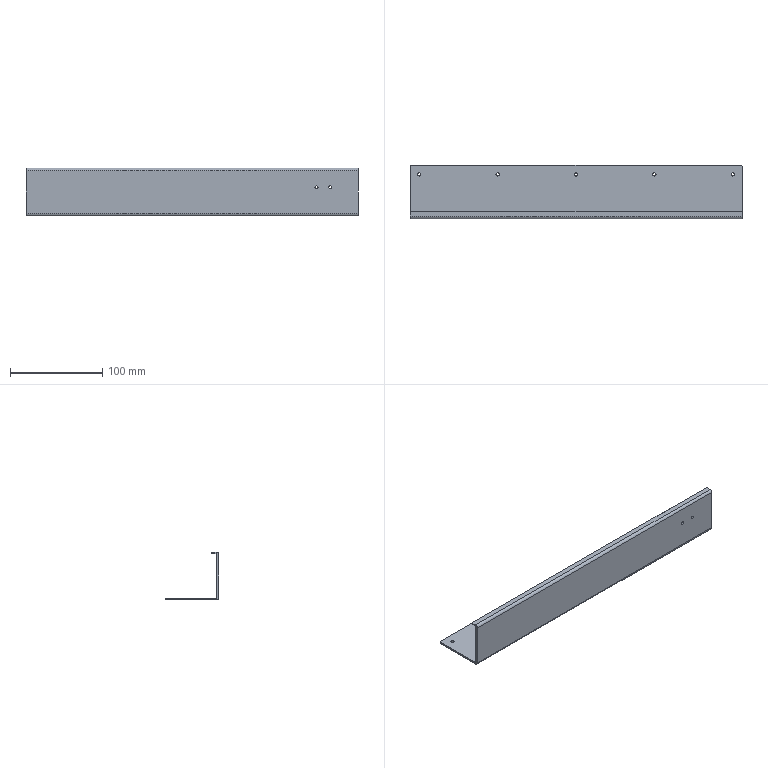Part | NX | features BREP 1 | 1 solid | 40 faces | box 360 x 58 x 52 mm | volume 80872 mm3 | plane 22 | cylinder 18 | commonest cylinder face diameters 3.5 x10 3.3 x4 1.473 x2 5.473 x2
STEP:
#1=CARTESIAN_POINT('',(135.,-2.,3.35));
#2=VERTEX_POINT('',#1);
#3=CARTESIAN_POINT('',(135.,-2.,6.65));
#4=VERTEX_POINT('',#3);
#5=CARTESIAN_POINT('',(135.,-2.,5.));
#6=DIRECTION('',(0.,1.,0.));
#7=DIRECTION('',(0.,0.,1.));
#8=AXIS2_PLACEMENT_3D('',#5,#6,#7);
#9=CIRCLE('',#8,1.65);
#10=EDGE_CURVE('',#2,#4,#9,.T.);
#11=ORIENTED_EDGE('',*,*,#10,.F.);
#12=CARTESIAN_POINT('',(135.,0.,3.35));
#13=VERTEX_POINT('',#12);
#14=CARTESIAN_POINT('',(135.,0.,3.35));
#15=DIRECTION('',(0.,1.,0.));
#16=VECTOR('',#15,1000.);
#17=LINE('',#14,#16);
#18=EDGE_CURVE('',#13,#2,#17,.F.);
#19=ORIENTED_EDGE('',*,*,#18,.F.);
#20=CARTESIAN_POINT('',(135.,0.,6.65));
#21=VERTEX_POINT('',#20);
#22=CARTESIAN_POINT('',(135.,0.,5.));
#23=DIRECTION('',(0.,1.,0.));
#24=DIRECTION('',(0.,0.,1.));
#25=AXIS2_PLACEMENT_3D('',#22,#23,#24);
#26=CIRCLE('',#25,1.65);
#27=EDGE_CURVE('',#13,#21,#26,.T.);
#28=ORIENTED_EDGE('',*,*,#27,.T.);
#29=CARTESIAN_POINT('',(135.,0.,6.65));
#30=DIRECTION('',(0.,1.,0.));
#31=VECTOR('',#30,1000.);
#32=LINE('',#29,#31);
#33=EDGE_CURVE('',#21,#4,#32,.F.);
#34=ORIENTED_EDGE('',*,*,#33,.T.);
#35=EDGE_LOOP('',(#11,#19,#28,#34));
#36=FACE_BOUND('',#35,.T.);
#37=CARTESIAN_POINT('',(135.,0.,5.));
#38=DIRECTION('',(0.,1.,0.));
#39=DIRECTION('',(0.,0.,1.));
#40=AXIS2_PLACEMENT_3D('',#37,#38,#39);
#41=CYLINDRICAL_SURFACE('',#40,1.65);
#42=ADVANCED_FACE('',(#36),#41,.F.);
#43=CARTESIAN_POINT('',(150.,-2.,3.35));
#44=VERTEX_POINT('',#43);
#45=CARTESIAN_POINT('',(150.,-2.,6.65));
#46=VERTEX_POINT('',#45);
#47=CARTESIAN_POINT('',(150.,-2.,5.));
#48=DIRECTION('',(0.,1.,0.));
#49=DIRECTION('',(0.,0.,1.));
#50=AXIS2_PLACEMENT_3D('',#47,#48,#49);
#51=CIRCLE('',#50,1.65);
#52=EDGE_CURVE('',#44,#46,#51,.T.);
#53=ORIENTED_EDGE('',*,*,#52,.F.);
#54=CARTESIAN_POINT('',(150.,0.,3.35));
#55=VERTEX_POINT('',#54);
#56=CARTESIAN_POINT('',(150.,0.,3.35));
#57=DIRECTION('',(0.,1.,0.));
#58=VECTOR('',#57,1000.);
#59=LINE('',#56,#58);
#60=EDGE_CURVE('',#55,#44,#59,.F.);
#61=ORIENTED_EDGE('',*,*,#60,.F.);
#62=CARTESIAN_POINT('',(150.,0.,6.65));
#63=VERTEX_POINT('',#62);
#64=CARTESIAN_POINT('',(150.,0.,5.));
#65=DIRECTION('',(0.,1.,0.));
#66=DIRECTION('',(0.,0.,1.));
#67=AXIS2_PLACEMENT_3D('',#64,#65,#66);
#68=CIRCLE('',#67,1.65);
#69=EDGE_CURVE('',#55,#63,#68,.T.);
#70=ORIENTED_EDGE('',*,*,#69,.T.);
#71=CARTESIAN_POINT('',(150.,0.,6.65));
#72=DIRECTION('',(0.,1.,0.));
#73=VECTOR('',#72,1000.);
#74=LINE('',#71,#73);
#75=EDGE_CURVE('',#63,#46,#74,.F.);
#76=ORIENTED_EDGE('',*,*,#75,.T.);
#77=EDGE_LOOP('',(#53,#61,#70,#76));
#78=FACE_BOUND('',#77,.T.);
#79=CARTESIAN_POINT('',(150.,0.,5.));
#80=DIRECTION('',(0.,1.,0.));
#81=DIRECTION('',(0.,0.,1.));
#82=AXIS2_PLACEMENT_3D('',#79,#80,#81);
#83=CYLINDRICAL_SURFACE('',#82,1.65);
#84=ADVANCED_FACE('',(#78),#83,.F.);
#85=CARTESIAN_POINT('',(-86.75,46.,-26.));
#86=VERTEX_POINT('',#85);
#87=CARTESIAN_POINT('',(-83.25,46.,-26.));
#88=VERTEX_POINT('',#87);
#89=CARTESIAN_POINT('',(-85.,46.,-26.));
#90=DIRECTION('',(0.,0.,1.));
#91=DIRECTION('',(0.,-1.,0.));
#92=AXIS2_PLACEMENT_3D('',#89,#90,#91);
#93=CIRCLE('',#92,1.75);
#94=EDGE_CURVE('',#86,#88,#93,.T.);
#95=ORIENTED_EDGE('',*,*,#94,.F.);
#96=CARTESIAN_POINT('',(-86.75,46.,-24.));
#97=VERTEX_POINT('',#96);
#98=CARTESIAN_POINT('',(-86.75,46.,-24.));
#99=DIRECTION('',(0.,0.,1.));
#100=VECTOR('',#99,1000.);
#101=LINE('',#98,#100);
#102=EDGE_CURVE('',#97,#86,#101,.F.);
#103=ORIENTED_EDGE('',*,*,#102,.F.);
#104=CARTESIAN_POINT('',(-83.25,46.,-24.));
#105=VERTEX_POINT('',#104);
#106=CARTESIAN_POINT('',(-85.,46.,-24.));
#107=DIRECTION('',(0.,0.,1.));
#108=DIRECTION('',(1.,0.,0.));
#109=AXIS2_PLACEMENT_3D('',#106,#107,#108);
#110=CIRCLE('',#109,1.75);
#111=EDGE_CURVE('',#97,#105,#110,.T.);
#112=ORIENTED_EDGE('',*,*,#111,.T.);
#113=CARTESIAN_POINT('',(-83.25,46.,-24.));
#114=DIRECTION('',(0.,0.,1.));
#115=VECTOR('',#114,1000.);
#116=LINE('',#113,#115);
#117=EDGE_CURVE('',#105,#88,#116,.F.);
#118=ORIENTED_EDGE('',*,*,#117,.T.);
#119=EDGE_LOOP('',(#95,#103,#112,#118));
#120=FACE_BOUND('',#119,.T.);
#121=CARTESIAN_POINT('',(-85.,46.,-24.));
#122=DIRECTION('',(0.,0.,1.));
#123=DIRECTION('',(1.,0.,0.));
#124=AXIS2_PLACEMENT_3D('',#121,#122,#123);
#125=CYLINDRICAL_SURFACE('',#124,1.75);
#126=ADVANCED_FACE('',(#120),#125,.F.);
#127=CARTESIAN_POINT('',(-1.75,46.,-26.));
#128=VERTEX_POINT('',#127);
#129=CARTESIAN_POINT('',(1.75,46.,-26.));
#130=VERTEX_POINT('',#129);
#131=CARTESIAN_POINT('',(0.,46.,-26.));
#132=DIRECTION('',(0.,0.,1.));
#133=DIRECTION('',(0.,-1.,0.));
#134=AXIS2_PLACEMENT_3D('',#131,#132,#133);
#135=CIRCLE('',#134,1.75);
#136=EDGE_CURVE('',#128,#130,#135,.T.);
#137=ORIENTED_EDGE('',*,*,#136,.F.);
#138=CARTESIAN_POINT('',(-1.75,46.,-24.));
#139=VERTEX_POINT('',#138);
#140=CARTESIAN_POINT('',(-1.75,46.,-24.));
#141=DIRECTION('',(0.,0.,1.));
#142=VECTOR('',#141,1000.);
#143=LINE('',#140,#142);
#144=EDGE_CURVE('',#139,#128,#143,.F.);
#145=ORIENTED_EDGE('',*,*,#144,.F.);
#146=CARTESIAN_POINT('',(1.75,46.,-24.));
#147=VERTEX_POINT('',#146);
#148=CARTESIAN_POINT('',(0.,46.,-24.));
#149=DIRECTION('',(0.,0.,1.));
#150=DIRECTION('',(1.,0.,0.));
#151=AXIS2_PLACEMENT_3D('',#148,#149,#150);
#152=CIRCLE('',#151,1.75);
#153=EDGE_CURVE('',#139,#147,#152,.T.);
#154=ORIENTED_EDGE('',*,*,#153,.T.);
#155=CARTESIAN_POINT('',(1.75,46.,-24.));
#156=DIRECTION('',(0.,0.,1.));
#157=VECTOR('',#156,1000.);
#158=LINE('',#155,#157);
#159=EDGE_CURVE('',#147,#130,#158,.F.);
#160=ORIENTED_EDGE('',*,*,#159,.T.);
#161=EDGE_LOOP('',(#137,#145,#154,#160));
#162=FACE_BOUND('',#161,.T.);
#163=CARTESIAN_POINT('',(0.,46.,-24.));
#164=DIRECTION('',(0.,0.,1.));
#165=DIRECTION('',(1.,0.,0.));
#166=AXIS2_PLACEMENT_3D('',#163,#164,#165);
#167=CYLINDRICAL_SURFACE('',#166,1.75);
#168=ADVANCED_FACE('',(#162),#167,.F.);
#169=CARTESIAN_POINT('',(83.25,46.,-26.));
#170=VERTEX_POINT('',#169);
#171=CARTESIAN_POINT('',(86.75,46.,-26.));
#172=VERTEX_POINT('',#171);
#173=CARTESIAN_POINT('',(85.,46.,-26.));
#174=DIRECTION('',(0.,0.,1.));
#175=DIRECTION('',(0.,-1.,0.));
#176=AXIS2_PLACEMENT_3D('',#173,#174,#175);
#177=CIRCLE('',#176,1.75);
#178=EDGE_CURVE('',#170,#172,#177,.T.);
#179=ORIENTED_EDGE('',*,*,#178,.F.);
#180=CARTESIAN_POINT('',(83.25,46.,-24.));
#181=VERTEX_POINT('',#180);
#182=CARTESIAN_POINT('',(83.25,46.,-24.));
#183=DIRECTION('',(0.,0.,1.));
#184=VECTOR('',#183,1000.);
#185=LINE('',#182,#184);
#186=EDGE_CURVE('',#181,#170,#185,.F.);
#187=ORIENTED_EDGE('',*,*,#186,.F.);
#188=CARTESIAN_POINT('',(86.75,46.,-24.));
#189=VERTEX_POINT('',#188);
#190=CARTESIAN_POINT('',(85.,46.,-24.));
#191=DIRECTION('',(0.,0.,1.));
#192=DIRECTION('',(1.,0.,0.));
#193=AXIS2_PLACEMENT_3D('',#190,#191,#192);
#194=CIRCLE('',#193,1.75);
#195=EDGE_CURVE('',#181,#189,#194,.T.);
#196=ORIENTED_EDGE('',*,*,#195,.T.);
#197=CARTESIAN_POINT('',(86.75,46.,-24.));
#198=DIRECTION('',(0.,0.,1.));
#199=VECTOR('',#198,1000.);
#200=LINE('',#197,#199);
#201=EDGE_CURVE('',#189,#172,#200,.F.);
#202=ORIENTED_EDGE('',*,*,#201,.T.);
#203=EDGE_LOOP('',(#179,#187,#196,#202));
#204=FACE_BOUND('',#203,.T.);
#205=CARTESIAN_POINT('',(85.,46.,-24.));
#206=DIRECTION('',(0.,0.,1.));
#207=DIRECTION('',(1.,0.,0.));
#208=AXIS2_PLACEMENT_3D('',#205,#206,#207);
#209=CYLINDRICAL_SURFACE('',#208,1.75);
#210=ADVANCED_FACE('',(#204),#209,.F.);
#211=CARTESIAN_POINT('',(168.25,46.,-26.));
#212=VERTEX_POINT('',#211);
#213=CARTESIAN_POINT('',(171.75,46.,-26.));
#214=VERTEX_POINT('',#213);
#215=CARTESIAN_POINT('',(170.,46.,-26.));
#216=DIRECTION('',(0.,0.,1.));
#217=DIRECTION('',(0.,-1.,0.));
#218=AXIS2_PLACEMENT_3D('',#215,#216,#217);
#219=CIRCLE('',#218,1.75);
#220=EDGE_CURVE('',#212,#214,#219,.T.);
#221=ORIENTED_EDGE('',*,*,#220,.F.);
#222=CARTESIAN_POINT('',(168.25,46.,-24.));
#223=VERTEX_POINT('',#222);
#224=CARTESIAN_POINT('',(168.25,46.,-24.));
#225=DIRECTION('',(0.,0.,1.));
#226=VECTOR('',#225,1000.);
#227=LINE('',#224,#226);
#228=EDGE_CURVE('',#223,#212,#227,.F.);
#229=ORIENTED_EDGE('',*,*,#228,.F.);
#230=CARTESIAN_POINT('',(171.75,46.,-24.));
#231=VERTEX_POINT('',#230);
#232=CARTESIAN_POINT('',(170.,46.,-24.));
#233=DIRECTION('',(0.,0.,1.));
#234=DIRECTION('',(1.,0.,0.));
#235=AXIS2_PLACEMENT_3D('',#232,#233,#234);
#236=CIRCLE('',#235,1.75);
#237=EDGE_CURVE('',#223,#231,#236,.T.);
#238=ORIENTED_EDGE('',*,*,#237,.T.);
#239=CARTESIAN_POINT('',(171.75,46.,-24.));
#240=DIRECTION('',(0.,0.,1.));
#241=VECTOR('',#240,1000.);
#242=LINE('',#239,#241);
#243=EDGE_CURVE('',#231,#214,#242,.F.);
#244=ORIENTED_EDGE('',*,*,#243,.T.);
#245=EDGE_LOOP('',(#221,#229,#238,#244));
#246=FACE_BOUND('',#245,.T.);
#247=CARTESIAN_POINT('',(170.,46.,-24.));
#248=DIRECTION('',(0.,0.,1.));
#249=DIRECTION('',(1.,0.,0.));
#250=AXIS2_PLACEMENT_3D('',#247,#248,#249);
#251=CYLINDRICAL_SURFACE('',#250,1.75);
#252=ADVANCED_FACE('',(#246),#251,.F.);
#253=CARTESIAN_POINT('',(-171.75,46.,-26.));
#254=VERTEX_POINT('',#253);
#255=CARTESIAN_POINT('',(-168.25,46.,-26.));
#256=VERTEX_POINT('',#255);
#257=CARTESIAN_POINT('',(-170.,46.,-26.));
#258=DIRECTION('',(0.,0.,1.));
#259=DIRECTION('',(0.,-1.,0.));
#260=AXIS2_PLACEMENT_3D('',#257,#258,#259);
#261=CIRCLE('',#260,1.75);
#262=EDGE_CURVE('',#254,#256,#261,.T.);
#263=ORIENTED_EDGE('',*,*,#262,.F.);
#264=CARTESIAN_POINT('',(-171.75,46.,-24.));
#265=VERTEX_POINT('',#264);
#266=CARTESIAN_POINT('',(-171.75,46.,-24.));
#267=DIRECTION('',(0.,0.,1.));
#268=VECTOR('',#267,1000.);
#269=LINE('',#266,#268);
#270=EDGE_CURVE('',#265,#254,#269,.F.);
#271=ORIENTED_EDGE('',*,*,#270,.F.);
#272=CARTESIAN_POINT('',(-168.25,46.,-24.));
#273=VERTEX_POINT('',#272);
#274=CARTESIAN_POINT('',(-170.,46.,-24.));
#275=DIRECTION('',(0.,0.,1.));
#276=DIRECTION('',(1.,0.,0.));
#277=AXIS2_PLACEMENT_3D('',#274,#275,#276);
#278=CIRCLE('',#277,1.75);
#279=EDGE_CURVE('',#265,#273,#278,.T.);
#280=ORIENTED_EDGE('',*,*,#279,.T.);
#281=CARTESIAN_POINT('',(-168.25,46.,-24.));
#282=DIRECTION('',(0.,0.,1.));
#283=VECTOR('',#282,1000.);
#284=LINE('',#281,#283);
#285=EDGE_CURVE('',#273,#256,#284,.F.);
#286=ORIENTED_EDGE('',*,*,#285,.T.);
#287=EDGE_LOOP('',(#263,#271,#280,#286));
#288=FACE_BOUND('',#287,.T.);
#289=CARTESIAN_POINT('',(-170.,46.,-24.));
#290=DIRECTION('',(0.,0.,1.));
#291=DIRECTION('',(1.,0.,0.));
#292=AXIS2_PLACEMENT_3D('',#289,#290,#291);
#293=CYLINDRICAL_SURFACE('',#292,1.75);
#294=ADVANCED_FACE('',(#288),#293,.F.);
#295=CARTESIAN_POINT('',(180.,-2.,23.263));
#296=VERTEX_POINT('',#295);
#297=CARTESIAN_POINT('',(-180.,-2.,23.263));
#298=VERTEX_POINT('',#297);
#299=CARTESIAN_POINT('',(180.,-2.,23.263));
#300=DIRECTION('',(-1.,0.,0.));
#301=VECTOR('',#300,1000.);
#302=LINE('',#299,#301);
#303=EDGE_CURVE('',#296,#298,#302,.T.);
#304=ORIENTED_EDGE('',*,*,#303,.T.);
#305=CARTESIAN_POINT('',(-180.,-2.,-23.263));
#306=VERTEX_POINT('',#305);
#307=CARTESIAN_POINT('',(-180.,-2.,-24.));
#308=DIRECTION('',(0.,0.,1.));
#309=VECTOR('',#308,1000.);
#310=LINE('',#307,#309);
#311=EDGE_CURVE('',#306,#298,#310,.T.);
#312=ORIENTED_EDGE('',*,*,#311,.F.);
#313=CARTESIAN_POINT('',(180.,-2.,-23.263));
#314=VERTEX_POINT('',#313);
#315=CARTESIAN_POINT('',(-180.,-2.,-23.263));
#316=DIRECTION('',(1.,0.,0.));
#317=VECTOR('',#316,1000.);
#318=LINE('',#315,#317);
#319=EDGE_CURVE('',#306,#314,#318,.T.);
#320=ORIENTED_EDGE('',*,*,#319,.T.);
#321=CARTESIAN_POINT('',(180.,-2.,-24.));
#322=DIRECTION('',(0.,0.,-1.));
#323=VECTOR('',#322,1000.);
#324=LINE('',#321,#323);
#325=EDGE_CURVE('',#296,#314,#324,.T.);
#326=ORIENTED_EDGE('',*,*,#325,.F.);
#327=EDGE_LOOP('',(#304,#312,#320,#326));
#328=FACE_BOUND('',#327,.T.);
#329=CARTESIAN_POINT('',(150.,-2.,5.));
#330=DIRECTION('',(0.,1.,0.));
#331=DIRECTION('',(0.,0.,1.));
#332=AXIS2_PLACEMENT_3D('',#329,#330,#331);
#333=CIRCLE('',#332,1.65);
#334=EDGE_CURVE('',#46,#44,#333,.T.);
#335=ORIENTED_EDGE('',*,*,#334,.T.);
#336=ORIENTED_EDGE('',*,*,#52,.T.);
#337=EDGE_LOOP('',(#335,#336));
#338=FACE_BOUND('',#337,.T.);
#339=CARTESIAN_POINT('',(135.,-2.,5.));
#340=DIRECTION('',(0.,1.,0.));
#341=DIRECTION('',(0.,0.,1.));
#342=AXIS2_PLACEMENT_3D('',#339,#340,#341);
#343=CIRCLE('',#342,1.65);
#344=EDGE_CURVE('',#4,#2,#343,.T.);
#345=ORIENTED_EDGE('',*,*,#344,.T.);
#346=ORIENTED_EDGE('',*,*,#10,.T.);
#347=EDGE_LOOP('',(#345,#346));
#348=FACE_BOUND('',#347,.T.);
#349=CARTESIAN_POINT('',(0.,-2.,0.));
#350=DIRECTION('',(0.,1.,0.));
#351=DIRECTION('',(1.,0.,0.));
#352=AXIS2_PLACEMENT_3D('',#349,#350,#351);
#353=PLANE('',#352);
#354=ADVANCED_FACE('',(#328,#338,#348),#353,.F.);
#355=CARTESIAN_POINT('',(-180.,0.,-23.263));
#356=VERTEX_POINT('',#355);
#357=CARTESIAN_POINT('',(-180.,0.,23.263));
#358=VERTEX_POINT('',#357);
#359=CARTESIAN_POINT('',(-180.,0.,-24.));
#360=DIRECTION('',(0.,0.,1.));
#361=VECTOR('',#360,1000.);
#362=LINE('',#359,#361);
#363=EDGE_CURVE('',#356,#358,#362,.T.);
#364=ORIENTED_EDGE('',*,*,#363,.T.);
#365=CARTESIAN_POINT('',(180.,0.,23.263));
#366=VERTEX_POINT('',#365);
#367=CARTESIAN_POINT('',(180.,0.,23.263));
#368=DIRECTION('',(-1.,0.,0.));
#369=VECTOR('',#368,1000.);
#370=LINE('',#367,#369);
#371=EDGE_CURVE('',#366,#358,#370,.T.);
#372=ORIENTED_EDGE('',*,*,#371,.F.);
#373=CARTESIAN_POINT('',(180.,0.,-23.263));
#374=VERTEX_POINT('',#373);
#375=CARTESIAN_POINT('',(180.,0.,-24.));
#376=DIRECTION('',(0.,0.,-1.));
#377=VECTOR('',#376,1000.);
#378=LINE('',#375,#377);
#379=EDGE_CURVE('',#366,#374,#378,.T.);
#380=ORIENTED_EDGE('',*,*,#379,.T.);
#381=CARTESIAN_POINT('',(-180.,0.,-23.263));
#382=DIRECTION('',(1.,0.,0.));
#383=VECTOR('',#382,1000.);
#384=LINE('',#381,#383);
#385=EDGE_CURVE('',#356,#374,#384,.T.);
#386=ORIENTED_EDGE('',*,*,#385,.F.);
#387=EDGE_LOOP('',(#364,#372,#380,#386));
#388=FACE_BOUND('',#387,.T.);
#389=CARTESIAN_POINT('',(150.,0.,5.));
#390=DIRECTION('',(0.,1.,0.));
#391=DIRECTION('',(0.,0.,1.));
#392=AXIS2_PLACEMENT_3D('',#389,#390,#391);
#393=CIRCLE('',#392,1.65);
#394=EDGE_CURVE('',#63,#55,#393,.T.);
#395=ORIENTED_EDGE('',*,*,#394,.F.);
#396=ORIENTED_EDGE('',*,*,#69,.F.);
#397=EDGE_LOOP('',(#395,#396));
#398=FACE_BOUND('',#397,.T.);
#399=CARTESIAN_POINT('',(135.,0.,5.));
#400=DIRECTION('',(0.,1.,0.));
#401=DIRECTION('',(0.,0.,1.));
#402=AXIS2_PLACEMENT_3D('',#399,#400,#401);
#403=CIRCLE('',#402,1.65);
#404=EDGE_CURVE('',#21,#13,#403,.T.);
#405=ORIENTED_EDGE('',*,*,#404,.F.);
#406=ORIENTED_EDGE('',*,*,#27,.F.);
#407=EDGE_LOOP('',(#405,#406));
#408=FACE_BOUND('',#407,.T.);
#409=CARTESIAN_POINT('',(0.,0.,0.));
#410=DIRECTION('',(0.,1.,0.));
#411=DIRECTION('',(1.,0.,0.));
#412=AXIS2_PLACEMENT_3D('',#409,#410,#411);
#413=PLANE('',#412);
#414=ADVANCED_FACE('',(#388,#398,#408),#413,.T.);
#415=ORIENTED_EDGE('',*,*,#379,.F.);
#416=CARTESIAN_POINT('',(180.,0.,23.263));
#417=DIRECTION('',(0.,-1.,0.));
#418=VECTOR('',#417,1000.);
#419=LINE('',#416,#418);
#420=EDGE_CURVE('',#366,#296,#419,.T.);
#421=ORIENTED_EDGE('',*,*,#420,.T.);
#422=ORIENTED_EDGE('',*,*,#325,.T.);
#423=CARTESIAN_POINT('',(180.,0.,-23.263));
#424=DIRECTION('',(0.,-1.,0.));
#425=VECTOR('',#424,1000.);
#426=LINE('',#423,#425);
#427=EDGE_CURVE('',#374,#314,#426,.T.);
#428=ORIENTED_EDGE('',*,*,#427,.F.);
#429=EDGE_LOOP('',(#415,#421,#422,#428));
#430=FACE_BOUND('',#429,.T.);
#431=CARTESIAN_POINT('',(180.,-2.,-24.));
#432=DIRECTION('',(1.,0.,0.));
#433=DIRECTION('',(0.,1.,0.));
#434=AXIS2_PLACEMENT_3D('',#431,#432,#433);
#435=PLANE('',#434);
#436=ADVANCED_FACE('',(#430),#435,.T.);
#437=CARTESIAN_POINT('',(-180.,0.,23.263));
#438=DIRECTION('',(0.,-1.,0.));
#439=VECTOR('',#438,1000.);
#440=LINE('',#437,#439);
#441=EDGE_CURVE('',#358,#298,#440,.T.);
#442=ORIENTED_EDGE('',*,*,#441,.F.);
#443=ORIENTED_EDGE('',*,*,#363,.F.);
#444=CARTESIAN_POINT('',(-180.,0.,-23.263));
#445=DIRECTION('',(0.,-1.,0.));
#446=VECTOR('',#445,1000.);
#447=LINE('',#444,#446);
#448=EDGE_CURVE('',#356,#306,#447,.T.);
#449=ORIENTED_EDGE('',*,*,#448,.T.);
#450=ORIENTED_EDGE('',*,*,#311,.T.);
#451=EDGE_LOOP('',(#442,#443,#449,#450));
#452=FACE_BOUND('',#451,.T.);
#453=CARTESIAN_POINT('',(-180.,-2.,-24.));
#454=DIRECTION('',(-1.,0.,0.));
#455=DIRECTION('',(0.,0.,1.));
#456=AXIS2_PLACEMENT_3D('',#453,#454,#455);
#457=PLANE('',#456);
#458=ADVANCED_FACE('',(#452),#457,.T.);
#459=CARTESIAN_POINT('',(180.,0.7366,-24.));
#460=VERTEX_POINT('',#459);
#461=CARTESIAN_POINT('',(180.,0.7366,-26.));
#462=VERTEX_POINT('',#461);
#463=CARTESIAN_POINT('',(180.,0.7366,-24.));
#464=DIRECTION('',(0.,0.,-1.));
#465=VECTOR('',#464,1000.);
#466=LINE('',#463,#465);
#467=EDGE_CURVE('',#460,#462,#466,.T.);
#468=ORIENTED_EDGE('',*,*,#467,.F.);
#469=CARTESIAN_POINT('',(180.,0.7366,-23.263));
#470=DIRECTION('',(1.,0.,0.));
#471=DIRECTION('',(0.,-1.,0.));
#472=AXIS2_PLACEMENT_3D('',#469,#470,#471);
#473=CIRCLE('',#472,0.7366);
#474=EDGE_CURVE('',#374,#460,#473,.T.);
#475=ORIENTED_EDGE('',*,*,#474,.F.);
#476=ORIENTED_EDGE('',*,*,#427,.T.);
#477=CARTESIAN_POINT('',(180.,0.7366,-23.263));
#478=DIRECTION('',(1.,0.,0.));
#479=DIRECTION('',(0.,-1.,0.));
#480=AXIS2_PLACEMENT_3D('',#477,#478,#479);
#481=CIRCLE('',#480,2.737);
#482=EDGE_CURVE('',#314,#462,#481,.T.);
#483=ORIENTED_EDGE('',*,*,#482,.T.);
#484=EDGE_LOOP('',(#468,#475,#476,#483));
#485=FACE_BOUND('',#484,.T.);
#486=CARTESIAN_POINT('',(180.,0.7366,-23.263));
#487=DIRECTION('',(1.,0.,0.));
#488=DIRECTION('',(0.,-1.,0.));
#489=AXIS2_PLACEMENT_3D('',#486,#487,#488);
#490=PLANE('',#489);
#491=ADVANCED_FACE('',(#485),#490,.T.);
#492=CARTESIAN_POINT('',(-180.,0.7366,-24.));
#493=VERTEX_POINT('',#492);
#494=CARTESIAN_POINT('',(-180.,0.7366,-23.263));
#495=DIRECTION('',(-1.,0.,0.));
#496=DIRECTION('',(0.,-1.,0.));
#497=AXIS2_PLACEMENT_3D('',#494,#495,#496);
#498=CIRCLE('',#497,0.7366);
#499=EDGE_CURVE('',#493,#356,#498,.T.);
#500=ORIENTED_EDGE('',*,*,#499,.F.);
#501=CARTESIAN_POINT('',(-180.,0.7366,-26.));
#502=VERTEX_POINT('',#501);
#503=CARTESIAN_POINT('',(-180.,0.7366,-24.));
#504=DIRECTION('',(0.,0.,-1.));
#505=VECTOR('',#504,1000.);
#506=LINE('',#503,#505);
#507=EDGE_CURVE('',#493,#502,#506,.T.);
#508=ORIENTED_EDGE('',*,*,#507,.T.);
#509=CARTESIAN_POINT('',(-180.,0.7366,-23.263));
#510=DIRECTION('',(-1.,0.,0.));
#511=DIRECTION('',(0.,-1.,0.));
#512=AXIS2_PLACEMENT_3D('',#509,#510,#511);
#513=CIRCLE('',#512,2.737);
#514=EDGE_CURVE('',#502,#306,#513,.T.);
#515=ORIENTED_EDGE('',*,*,#514,.T.);
#516=ORIENTED_EDGE('',*,*,#448,.F.);
#517=EDGE_LOOP('',(#500,#508,#515,#516));
#518=FACE_BOUND('',#517,.T.);
#519=CARTESIAN_POINT('',(-180.,0.7366,-23.263));
#520=DIRECTION('',(1.,0.,0.));
#521=DIRECTION('',(0.,-1.,0.));
#522=AXIS2_PLACEMENT_3D('',#519,#520,#521);
#523=PLANE('',#522);
#524=ADVANCED_FACE('',(#518),#523,.F.);
#525=ORIENTED_EDGE('',*,*,#319,.F.);
#526=ORIENTED_EDGE('',*,*,#514,.F.);
#527=CARTESIAN_POINT('',(0.,0.7366,-26.));
#528=DIRECTION('',(1.,0.,0.));
#529=VECTOR('',#528,1000.);
#530=LINE('',#527,#529);
#531=EDGE_CURVE('',#502,#462,#530,.T.);
#532=ORIENTED_EDGE('',*,*,#531,.T.);
#533=ORIENTED_EDGE('',*,*,#482,.F.);
#534=EDGE_LOOP('',(#525,#526,#532,#533));
#535=FACE_BOUND('',#534,.T.);
#536=CARTESIAN_POINT('',(-180.,0.7366,-23.263));
#537=DIRECTION('',(-1.,0.,0.));
#538=DIRECTION('',(0.,0.,-1.));
#539=AXIS2_PLACEMENT_3D('',#536,#537,#538);
#540=CYLINDRICAL_SURFACE('',#539,2.737);
#541=ADVANCED_FACE('',(#535),#540,.T.);
#542=ORIENTED_EDGE('',*,*,#385,.T.);
#543=ORIENTED_EDGE('',*,*,#474,.T.);
#544=CARTESIAN_POINT('',(180.,0.7366,-24.));
#545=DIRECTION('',(-1.,0.,0.));
#546=VECTOR('',#545,1000.);
#547=LINE('',#544,#546);
#548=EDGE_CURVE('',#460,#493,#547,.T.);
#549=ORIENTED_EDGE('',*,*,#548,.T.);
#550=ORIENTED_EDGE('',*,*,#499,.T.);
#551=EDGE_LOOP('',(#542,#543,#549,#550));
#552=FACE_BOUND('',#551,.T.);
#553=CARTESIAN_POINT('',(-180.,0.7366,-23.263));
#554=DIRECTION('',(-1.,0.,0.));
#555=DIRECTION('',(0.,0.,-1.));
#556=AXIS2_PLACEMENT_3D('',#553,#554,#555);
#557=CYLINDRICAL_SURFACE('',#556,0.7366);
#558=ADVANCED_FACE('',(#552),#557,.F.);
#559=CARTESIAN_POINT('',(180.,55.,-26.));
#560=VERTEX_POINT('',#559);
#561=CARTESIAN_POINT('',(180.,0.,-26.));
#562=DIRECTION('',(0.,-1.,0.));
#563=VECTOR('',#562,1000.);
#564=LINE('',#561,#563);
#565=EDGE_CURVE('',#560,#462,#564,.T.);
#566=ORIENTED_EDGE('',*,*,#565,.F.);
#567=CARTESIAN_POINT('',(180.,55.,-24.));
#568=VERTEX_POINT('',#567);
#569=CARTESIAN_POINT('',(180.,55.,-26.));
#570=DIRECTION('',(0.,0.,1.));
#571=VECTOR('',#570,1000.);
#572=LINE('',#569,#571);
#573=EDGE_CURVE('',#560,#568,#572,.T.);
#574=ORIENTED_EDGE('',*,*,#573,.T.);
#575=CARTESIAN_POINT('',(180.,0.,-24.));
#576=DIRECTION('',(0.,-1.,0.));
#577=VECTOR('',#576,1000.);
#578=LINE('',#575,#577);
#579=EDGE_CURVE('',#568,#460,#578,.T.);
#580=ORIENTED_EDGE('',*,*,#579,.T.);
#581=ORIENTED_EDGE('',*,*,#467,.T.);
#582=EDGE_LOOP('',(#566,#574,#580,#581));
#583=FACE_BOUND('',#582,.T.);
#584=CARTESIAN_POINT('',(180.,0.,-26.));
#585=DIRECTION('',(-1.,0.,0.));
#586=DIRECTION('',(0.,0.,1.));
#587=AXIS2_PLACEMENT_3D('',#584,#585,#586);
#588=PLANE('',#587);
#589=ADVANCED_FACE('',(#583),#588,.F.);
#590=CARTESIAN_POINT('',(-180.,55.,-24.));
#591=VERTEX_POINT('',#590);
#592=CARTESIAN_POINT('',(-180.,56.,-24.));
#593=DIRECTION('',(0.,1.,0.));
#594=VECTOR('',#593,1000.);
#595=LINE('',#592,#594);
#596=EDGE_CURVE('',#493,#591,#595,.T.);
#597=ORIENTED_EDGE('',*,*,#596,.T.);
#598=CARTESIAN_POINT('',(-180.,55.,-26.));
#599=VERTEX_POINT('',#598);
#600=CARTESIAN_POINT('',(-180.,55.,-26.));
#601=DIRECTION('',(0.,0.,-1.));
#602=VECTOR('',#601,1000.);
#603=LINE('',#600,#602);
#604=EDGE_CURVE('',#591,#599,#603,.T.);
#605=ORIENTED_EDGE('',*,*,#604,.T.);
#606=CARTESIAN_POINT('',(-180.,56.,-26.));
#607=DIRECTION('',(0.,1.,0.));
#608=VECTOR('',#607,1000.);
#609=LINE('',#606,#608);
#610=EDGE_CURVE('',#502,#599,#609,.T.);
#611=ORIENTED_EDGE('',*,*,#610,.F.);
#612=ORIENTED_EDGE('',*,*,#507,.F.);
#613=EDGE_LOOP('',(#597,#605,#611,#612));
#614=FACE_BOUND('',#613,.T.);
#615=CARTESIAN_POINT('',(-180.,56.,-26.));
#616=DIRECTION('',(1.,0.,0.));
#617=DIRECTION('',(0.,1.,0.));
#618=AXIS2_PLACEMENT_3D('',#615,#616,#617);
#619=PLANE('',#618);
#620=ADVANCED_FACE('',(#614),#619,.F.);
#621=ORIENTED_EDGE('',*,*,#610,.T.);
#622=CARTESIAN_POINT('',(-179.,56.,-26.));
#623=VERTEX_POINT('',#622);
#624=CARTESIAN_POINT('',(-179.,56.,-26.));
#625=DIRECTION('',(0.7071,0.7071,0.));
#626=VECTOR('',#625,1000.);
#627=LINE('',#624,#626);
#628=EDGE_CURVE('',#599,#623,#627,.T.);
#629=ORIENTED_EDGE('',*,*,#628,.T.);
#630=CARTESIAN_POINT('',(179.,56.,-26.));
#631=VERTEX_POINT('',#630);
#632=CARTESIAN_POINT('',(180.,56.,-26.));
#633=DIRECTION('',(1.,0.,0.));
#634=VECTOR('',#633,1000.);
#635=LINE('',#632,#634);
#636=EDGE_CURVE('',#623,#631,#635,.T.);
#637=ORIENTED_EDGE('',*,*,#636,.T.);
#638=CARTESIAN_POINT('',(180.,55.,-26.));
#639=DIRECTION('',(0.7071,-0.7071,0.));
#640=VECTOR('',#639,1000.);
#641=LINE('',#638,#640);
#642=EDGE_CURVE('',#631,#560,#641,.T.);
#643=ORIENTED_EDGE('',*,*,#642,.T.);
#644=ORIENTED_EDGE('',*,*,#565,.T.);
#645=ORIENTED_EDGE('',*,*,#531,.F.);
#646=EDGE_LOOP('',(#621,#629,#637,#643,#644,#645));
#647=FACE_BOUND('',#646,.T.);
#648=CARTESIAN_POINT('',(-85.,46.,-26.));
#649=DIRECTION('',(0.,0.,1.));
#650=DIRECTION('',(0.,-1.,0.));
#651=AXIS2_PLACEMENT_3D('',#648,#649,#650);
#652=CIRCLE('',#651,1.75);
#653=EDGE_CURVE('',#88,#86,#652,.T.);
#654=ORIENTED_EDGE('',*,*,#653,.T.);
#655=ORIENTED_EDGE('',*,*,#94,.T.);
#656=EDGE_LOOP('',(#654,#655));
#657=FACE_BOUND('',#656,.T.);
#658=CARTESIAN_POINT('',(0.,46.,-26.));
#659=DIRECTION('',(0.,0.,1.));
#660=DIRECTION('',(0.,-1.,0.));
#661=AXIS2_PLACEMENT_3D('',#658,#659,#660);
#662=CIRCLE('',#661,1.75);
#663=EDGE_CURVE('',#130,#128,#662,.T.);
#664=ORIENTED_EDGE('',*,*,#663,.T.);
#665=ORIENTED_EDGE('',*,*,#136,.T.);
#666=EDGE_LOOP('',(#664,#665));
#667=FACE_BOUND('',#666,.T.);
#668=CARTESIAN_POINT('',(85.,46.,-26.));
#669=DIRECTION('',(0.,0.,1.));
#670=DIRECTION('',(0.,-1.,0.));
#671=AXIS2_PLACEMENT_3D('',#668,#669,#670);
#672=CIRCLE('',#671,1.75);
#673=EDGE_CURVE('',#172,#170,#672,.T.);
#674=ORIENTED_EDGE('',*,*,#673,.T.);
#675=ORIENTED_EDGE('',*,*,#178,.T.);
#676=EDGE_LOOP('',(#674,#675));
#677=FACE_BOUND('',#676,.T.);
#678=CARTESIAN_POINT('',(170.,46.,-26.));
#679=DIRECTION('',(0.,0.,1.));
#680=DIRECTION('',(0.,-1.,0.));
#681=AXIS2_PLACEMENT_3D('',#678,#679,#680);
#682=CIRCLE('',#681,1.75);
#683=EDGE_CURVE('',#214,#212,#682,.T.);
#684=ORIENTED_EDGE('',*,*,#683,.T.);
#685=ORIENTED_EDGE('',*,*,#220,.T.);
#686=EDGE_LOOP('',(#684,#685));
#687=FACE_BOUND('',#686,.T.);
#688=CARTESIAN_POINT('',(-170.,46.,-26.));
#689=DIRECTION('',(0.,0.,1.));
#690=DIRECTION('',(0.,-1.,0.));
#691=AXIS2_PLACEMENT_3D('',#688,#689,#690);
#692=CIRCLE('',#691,1.75);
#693=EDGE_CURVE('',#256,#254,#692,.T.);
#694=ORIENTED_EDGE('',*,*,#693,.T.);
#695=ORIENTED_EDGE('',*,*,#262,.T.);
#696=EDGE_LOOP('',(#694,#695));
#697=FACE_BOUND('',#696,.T.);
#698=CARTESIAN_POINT('',(0.,0.,-26.));
#699=DIRECTION('',(0.,0.,1.));
#700=DIRECTION('',(0.,-1.,0.));
#701=AXIS2_PLACEMENT_3D('',#698,#699,#700);
#702=PLANE('',#701);
#703=ADVANCED_FACE('',(#647,#657,#667,#677,#687,#697),#702,.F.);
#704=CARTESIAN_POINT('',(-179.,56.,-24.));
#705=VERTEX_POINT('',#704);
#706=CARTESIAN_POINT('',(179.,56.,-24.));
#707=VERTEX_POINT('',#706);
#708=CARTESIAN_POINT('',(180.,56.,-24.));
#709=DIRECTION('',(1.,0.,0.));
#710=VECTOR('',#709,1000.);
#711=LINE('',#708,#710);
#712=EDGE_CURVE('',#705,#707,#711,.T.);
#713=ORIENTED_EDGE('',*,*,#712,.F.);
#714=CARTESIAN_POINT('',(-117.5,117.5,-24.));
#715=DIRECTION('',(-0.7071,-0.7071,0.));
#716=VECTOR('',#715,1000.);
#717=LINE('',#714,#716);
#718=EDGE_CURVE('',#705,#591,#717,.T.);
#719=ORIENTED_EDGE('',*,*,#718,.T.);
#720=ORIENTED_EDGE('',*,*,#596,.F.);
#721=ORIENTED_EDGE('',*,*,#548,.F.);
#722=ORIENTED_EDGE('',*,*,#579,.F.);
#723=CARTESIAN_POINT('',(117.5,117.5,-24.));
#724=DIRECTION('',(-0.7071,0.7071,0.));
#725=VECTOR('',#724,1000.);
#726=LINE('',#723,#725);
#727=EDGE_CURVE('',#568,#707,#726,.T.);
#728=ORIENTED_EDGE('',*,*,#727,.T.);
#729=EDGE_LOOP('',(#713,#719,#720,#721,#722,#728));
#730=FACE_BOUND('',#729,.T.);
#731=CARTESIAN_POINT('',(-85.,46.,-24.));
#732=DIRECTION('',(0.,0.,1.));
#733=DIRECTION('',(1.,0.,0.));
#734=AXIS2_PLACEMENT_3D('',#731,#732,#733);
#735=CIRCLE('',#734,1.75);
#736=EDGE_CURVE('',#105,#97,#735,.T.);
#737=ORIENTED_EDGE('',*,*,#736,.F.);
#738=ORIENTED_EDGE('',*,*,#111,.F.);
#739=EDGE_LOOP('',(#737,#738));
#740=FACE_BOUND('',#739,.T.);
#741=CARTESIAN_POINT('',(0.,46.,-24.));
#742=DIRECTION('',(0.,0.,1.));
#743=DIRECTION('',(1.,0.,0.));
#744=AXIS2_PLACEMENT_3D('',#741,#742,#743);
#745=CIRCLE('',#744,1.75);
#746=EDGE_CURVE('',#147,#139,#745,.T.);
#747=ORIENTED_EDGE('',*,*,#746,.F.);
#748=ORIENTED_EDGE('',*,*,#153,.F.);
#749=EDGE_LOOP('',(#747,#748));
#750=FACE_BOUND('',#749,.T.);
#751=CARTESIAN_POINT('',(85.,46.,-24.));
#752=DIRECTION('',(0.,0.,1.));
#753=DIRECTION('',(1.,0.,0.));
#754=AXIS2_PLACEMENT_3D('',#751,#752,#753);
#755=CIRCLE('',#754,1.75);
#756=EDGE_CURVE('',#189,#181,#755,.T.);
#757=ORIENTED_EDGE('',*,*,#756,.F.);
#758=ORIENTED_EDGE('',*,*,#195,.F.);
#759=EDGE_LOOP('',(#757,#758));
#760=FACE_BOUND('',#759,.T.);
#761=CARTESIAN_POINT('',(170.,46.,-24.));
#762=DIRECTION('',(0.,0.,1.));
#763=DIRECTION('',(1.,0.,0.));
#764=AXIS2_PLACEMENT_3D('',#761,#762,#763);
#765=CIRCLE('',#764,1.75);
#766=EDGE_CURVE('',#231,#223,#765,.T.);
#767=ORIENTED_EDGE('',*,*,#766,.F.);
#768=ORIENTED_EDGE('',*,*,#237,.F.);
#769=EDGE_LOOP('',(#767,#768));
#770=FACE_BOUND('',#769,.T.);
#771=CARTESIAN_POINT('',(-170.,46.,-24.));
#772=DIRECTION('',(0.,0.,1.));
#773=DIRECTION('',(1.,0.,0.));
#774=AXIS2_PLACEMENT_3D('',#771,#772,#773);
#775=CIRCLE('',#774,1.75);
#776=EDGE_CURVE('',#273,#265,#775,.T.);
#777=ORIENTED_EDGE('',*,*,#776,.F.);
#778=ORIENTED_EDGE('',*,*,#279,.F.);
#779=EDGE_LOOP('',(#777,#778));
#780=FACE_BOUND('',#779,.T.);
#781=CARTESIAN_POINT('',(0.,0.,-24.));
#782=DIRECTION('',(0.,0.,1.));
#783=DIRECTION('',(0.,-1.,0.));
#784=AXIS2_PLACEMENT_3D('',#781,#782,#783);
#785=PLANE('',#784);
#786=ADVANCED_FACE('',(#730,#740,#750,#760,#770,#780),#785,.T.);
#787=ORIENTED_EDGE('',*,*,#636,.F.);
#788=CARTESIAN_POINT('',(-179.,56.,-26.));
#789=DIRECTION('',(0.,0.,1.));
#790=VECTOR('',#789,1000.);
#791=LINE('',#788,#790);
#792=EDGE_CURVE('',#623,#705,#791,.T.);
#793=ORIENTED_EDGE('',*,*,#792,.T.);
#794=ORIENTED_EDGE('',*,*,#712,.T.);
#795=CARTESIAN_POINT('',(179.,56.,-26.));
#796=DIRECTION('',(0.,0.,-1.));
#797=VECTOR('',#796,1000.);
#798=LINE('',#795,#797);
#799=EDGE_CURVE('',#707,#631,#798,.T.);
#800=ORIENTED_EDGE('',*,*,#799,.T.);
#801=EDGE_LOOP('',(#787,#793,#794,#800));
#802=FACE_BOUND('',#801,.T.);
#803=CARTESIAN_POINT('',(180.,56.,-26.));
#804=DIRECTION('',(0.,-1.,0.));
#805=DIRECTION('',(-1.,0.,0.));
#806=AXIS2_PLACEMENT_3D('',#803,#804,#805);
#807=PLANE('',#806);
#808=ADVANCED_FACE('',(#802),#807,.F.);
#809=ORIENTED_EDGE('',*,*,#270,.T.);
#810=ORIENTED_EDGE('',*,*,#693,.F.);
#811=ORIENTED_EDGE('',*,*,#285,.F.);
#812=ORIENTED_EDGE('',*,*,#776,.T.);
#813=EDGE_LOOP('',(#809,#810,#811,#812));
#814=FACE_BOUND('',#813,.T.);
#815=CARTESIAN_POINT('',(-170.,46.,-24.));
#816=DIRECTION('',(0.,0.,1.));
#817=DIRECTION('',(1.,0.,0.));
#818=AXIS2_PLACEMENT_3D('',#815,#816,#817);
#819=CYLINDRICAL_SURFACE('',#818,1.75);
#820=ADVANCED_FACE('',(#814),#819,.F.);
#821=ORIENTED_EDGE('',*,*,#228,.T.);
#822=ORIENTED_EDGE('',*,*,#683,.F.);
#823=ORIENTED_EDGE('',*,*,#243,.F.);
#824=ORIENTED_EDGE('',*,*,#766,.T.);
#825=EDGE_LOOP('',(#821,#822,#823,#824));
#826=FACE_BOUND('',#825,.T.);
#827=CARTESIAN_POINT('',(170.,46.,-24.));
#828=DIRECTION('',(0.,0.,1.));
#829=DIRECTION('',(1.,0.,0.));
#830=AXIS2_PLACEMENT_3D('',#827,#828,#829);
#831=CYLINDRICAL_SURFACE('',#830,1.75);
#832=ADVANCED_FACE('',(#826),#831,.F.);
#833=ORIENTED_EDGE('',*,*,#186,.T.);
#834=ORIENTED_EDGE('',*,*,#673,.F.);
#835=ORIENTED_EDGE('',*,*,#201,.F.);
#836=ORIENTED_EDGE('',*,*,#756,.T.);
#837=EDGE_LOOP('',(#833,#834,#835,#836));
#838=FACE_BOUND('',#837,.T.);
#839=CARTESIAN_POINT('',(85.,46.,-24.));
#840=DIRECTION('',(0.,0.,1.));
#841=DIRECTION('',(1.,0.,0.));
#842=AXIS2_PLACEMENT_3D('',#839,#840,#841);
#843=CYLINDRICAL_SURFACE('',#842,1.75);
#844=ADVANCED_FACE('',(#838),#843,.F.);
#845=ORIENTED_EDGE('',*,*,#144,.T.);
#846=ORIENTED_EDGE('',*,*,#663,.F.);
#847=ORIENTED_EDGE('',*,*,#159,.F.);
#848=ORIENTED_EDGE('',*,*,#746,.T.);
#849=EDGE_LOOP('',(#845,#846,#847,#848));
#850=FACE_BOUND('',#849,.T.);
#851=CARTESIAN_POINT('',(0.,46.,-24.));
#852=DIRECTION('',(0.,0.,1.));
#853=DIRECTION('',(1.,0.,0.));
#854=AXIS2_PLACEMENT_3D('',#851,#852,#853);
#855=CYLINDRICAL_SURFACE('',#854,1.75);
#856=ADVANCED_FACE('',(#850),#855,.F.);
#857=ORIENTED_EDGE('',*,*,#102,.T.);
#858=ORIENTED_EDGE('',*,*,#653,.F.);
#859=ORIENTED_EDGE('',*,*,#117,.F.);
#860=ORIENTED_EDGE('',*,*,#736,.T.);
#861=EDGE_LOOP('',(#857,#858,#859,#860));
#862=FACE_BOUND('',#861,.T.);
#863=CARTESIAN_POINT('',(-85.,46.,-24.));
#864=DIRECTION('',(0.,0.,1.));
#865=DIRECTION('',(1.,0.,0.));
#866=AXIS2_PLACEMENT_3D('',#863,#864,#865);
#867=CYLINDRICAL_SURFACE('',#866,1.75);
#868=ADVANCED_FACE('',(#862),#867,.F.);
#869=ORIENTED_EDGE('',*,*,#60,.T.);
#870=ORIENTED_EDGE('',*,*,#334,.F.);
#871=ORIENTED_EDGE('',*,*,#75,.F.);
#872=ORIENTED_EDGE('',*,*,#394,.T.);
#873=EDGE_LOOP('',(#869,#870,#871,#872));
#874=FACE_BOUND('',#873,.T.);
#875=CARTESIAN_POINT('',(150.,0.,5.));
#876=DIRECTION('',(0.,1.,0.));
#877=DIRECTION('',(0.,0.,1.));
#878=AXIS2_PLACEMENT_3D('',#875,#876,#877);
#879=CYLINDRICAL_SURFACE('',#878,1.65);
#880=ADVANCED_FACE('',(#874),#879,.F.);
#881=ORIENTED_EDGE('',*,*,#18,.T.);
#882=ORIENTED_EDGE('',*,*,#344,.F.);
#883=ORIENTED_EDGE('',*,*,#33,.F.);
#884=ORIENTED_EDGE('',*,*,#404,.T.);
#885=EDGE_LOOP('',(#881,#882,#883,#884));
#886=FACE_BOUND('',#885,.T.);
#887=CARTESIAN_POINT('',(135.,0.,5.));
#888=DIRECTION('',(0.,1.,0.));
#889=DIRECTION('',(0.,0.,1.));
#890=AXIS2_PLACEMENT_3D('',#887,#888,#889);
#891=CYLINDRICAL_SURFACE('',#890,1.65);
#892=ADVANCED_FACE('',(#886),#891,.F.);
#893=CARTESIAN_POINT('',(-180.,0.7366,24.));
#894=VERTEX_POINT('',#893);
#895=CARTESIAN_POINT('',(-180.,0.7366,26.));
#896=VERTEX_POINT('',#895);
#897=CARTESIAN_POINT('',(-180.,0.7366,24.));
#898=DIRECTION('',(0.,0.,1.));
#899=VECTOR('',#898,1000.);
#900=LINE('',#897,#899);
#901=EDGE_CURVE('',#894,#896,#900,.T.);
#902=ORIENTED_EDGE('',*,*,#901,.F.);
#903=CARTESIAN_POINT('',(-180.,0.7366,23.263));
#904=DIRECTION('',(-1.,0.,0.));
#905=DIRECTION('',(0.,0.,-1.));
#906=AXIS2_PLACEMENT_3D('',#903,#904,#905);
#907=CIRCLE('',#906,0.7366);
#908=EDGE_CURVE('',#358,#894,#907,.T.);
#909=ORIENTED_EDGE('',*,*,#908,.F.);
#910=ORIENTED_EDGE('',*,*,#441,.T.);
#911=CARTESIAN_POINT('',(-180.,0.7366,23.263));
#912=DIRECTION('',(-1.,0.,0.));
#913=DIRECTION('',(0.,0.,-1.));
#914=AXIS2_PLACEMENT_3D('',#911,#912,#913);
#915=CIRCLE('',#914,2.737);
#916=EDGE_CURVE('',#298,#896,#915,.T.);
#917=ORIENTED_EDGE('',*,*,#916,.T.);
#918=EDGE_LOOP('',(#902,#909,#910,#917));
#919=FACE_BOUND('',#918,.T.);
#920=CARTESIAN_POINT('',(-180.,0.7366,23.263));
#921=DIRECTION('',(-1.,0.,0.));
#922=DIRECTION('',(0.,0.,1.));
#923=AXIS2_PLACEMENT_3D('',#920,#921,#922);
#924=PLANE('',#923);
#925=ADVANCED_FACE('',(#919),#924,.T.);
#926=CARTESIAN_POINT('',(180.,0.7366,24.));
#927=VERTEX_POINT('',#926);
#928=CARTESIAN_POINT('',(180.,0.7366,23.263));
#929=DIRECTION('',(1.,0.,0.));
#930=DIRECTION('',(0.,0.,-1.));
#931=AXIS2_PLACEMENT_3D('',#928,#929,#930);
#932=CIRCLE('',#931,0.7366);
#933=EDGE_CURVE('',#927,#366,#932,.T.);
#934=ORIENTED_EDGE('',*,*,#933,.F.);
#935=CARTESIAN_POINT('',(180.,0.7366,26.));
#936=VERTEX_POINT('',#935);
#937=CARTESIAN_POINT('',(180.,0.7366,24.));
#938=DIRECTION('',(0.,0.,1.));
#939=VECTOR('',#938,1000.);
#940=LINE('',#937,#939);
#941=EDGE_CURVE('',#927,#936,#940,.T.);
#942=ORIENTED_EDGE('',*,*,#941,.T.);
#943=CARTESIAN_POINT('',(180.,0.7366,23.263));
#944=DIRECTION('',(1.,0.,0.));
#945=DIRECTION('',(0.,0.,-1.));
#946=AXIS2_PLACEMENT_3D('',#943,#944,#945);
#947=CIRCLE('',#946,2.737);
#948=EDGE_CURVE('',#936,#296,#947,.T.);
#949=ORIENTED_EDGE('',*,*,#948,.T.);
#950=ORIENTED_EDGE('',*,*,#420,.F.);
#951=EDGE_LOOP('',(#934,#942,#949,#950));
#952=FACE_BOUND('',#951,.T.);
#953=CARTESIAN_POINT('',(180.,0.7366,23.263));
#954=DIRECTION('',(-1.,0.,0.));
#955=DIRECTION('',(0.,0.,1.));
#956=AXIS2_PLACEMENT_3D('',#953,#954,#955);
#957=PLANE('',#956);
#958=ADVANCED_FACE('',(#952),#957,.F.);
#959=ORIENTED_EDGE('',*,*,#303,.F.);
#960=ORIENTED_EDGE('',*,*,#948,.F.);
#961=CARTESIAN_POINT('',(0.,0.7366,26.));
#962=DIRECTION('',(1.,0.,0.));
#963=VECTOR('',#962,1000.);
#964=LINE('',#961,#963);
#965=EDGE_CURVE('',#896,#936,#964,.T.);
#966=ORIENTED_EDGE('',*,*,#965,.F.);
#967=ORIENTED_EDGE('',*,*,#916,.F.);
#968=EDGE_LOOP('',(#959,#960,#966,#967));
#969=FACE_BOUND('',#968,.T.);
#970=CARTESIAN_POINT('',(180.,0.7366,23.263));
#971=DIRECTION('',(1.,0.,0.));
#972=DIRECTION('',(0.,0.,1.));
#973=AXIS2_PLACEMENT_3D('',#970,#971,#972);
#974=CYLINDRICAL_SURFACE('',#973,2.737);
#975=ADVANCED_FACE('',(#969),#974,.T.);
#976=ORIENTED_EDGE('',*,*,#371,.T.);
#977=ORIENTED_EDGE('',*,*,#908,.T.);
#978=CARTESIAN_POINT('',(-180.,0.7366,24.));
#979=DIRECTION('',(1.,0.,0.));
#980=VECTOR('',#979,1000.);
#981=LINE('',#978,#980);
#982=EDGE_CURVE('',#894,#927,#981,.T.);
#983=ORIENTED_EDGE('',*,*,#982,.T.);
#984=ORIENTED_EDGE('',*,*,#933,.T.);
#985=EDGE_LOOP('',(#976,#977,#983,#984));
#986=FACE_BOUND('',#985,.T.);
#987=CARTESIAN_POINT('',(180.,0.7366,23.263));
#988=DIRECTION('',(1.,0.,0.));
#989=DIRECTION('',(0.,0.,1.));
#990=AXIS2_PLACEMENT_3D('',#987,#988,#989);
#991=CYLINDRICAL_SURFACE('',#990,0.7366);
#992=ADVANCED_FACE('',(#986),#991,.F.);
#993=CARTESIAN_POINT('',(180.,5.,24.));
#994=VERTEX_POINT('',#993);
#995=CARTESIAN_POINT('',(180.,0.,24.));
#996=DIRECTION('',(0.,-1.,0.));
#997=VECTOR('',#996,1000.);
#998=LINE('',#995,#997);
#999=EDGE_CURVE('',#994,#927,#998,.T.);
#1000=ORIENTED_EDGE('',*,*,#999,.F.);
#1001=CARTESIAN_POINT('',(180.,5.,26.));
#1002=VERTEX_POINT('',#1001);
#1003=CARTESIAN_POINT('',(180.,5.,26.));
#1004=DIRECTION('',(0.,0.,1.));
#1005=VECTOR('',#1004,1000.);
#1006=LINE('',#1003,#1005);
#1007=EDGE_CURVE('',#994,#1002,#1006,.T.);
#1008=ORIENTED_EDGE('',*,*,#1007,.T.);
#1009=CARTESIAN_POINT('',(180.,0.,26.));
#1010=DIRECTION('',(0.,-1.,0.));
#1011=VECTOR('',#1010,1000.);
#1012=LINE('',#1009,#1011);
#1013=EDGE_CURVE('',#1002,#936,#1012,.T.);
#1014=ORIENTED_EDGE('',*,*,#1013,.T.);
#1015=ORIENTED_EDGE('',*,*,#941,.F.);
#1016=EDGE_LOOP('',(#1000,#1008,#1014,#1015));
#1017=FACE_BOUND('',#1016,.T.);
#1018=CARTESIAN_POINT('',(180.,0.,26.));
#1019=DIRECTION('',(1.,0.,0.));
#1020=DIRECTION('',(0.,1.,0.));
#1021=AXIS2_PLACEMENT_3D('',#1018,#1019,#1020);
#1022=PLANE('',#1021);
#1023=ADVANCED_FACE('',(#1017),#1022,.T.);
#1024=CARTESIAN_POINT('',(-180.,5.,26.));
#1025=VERTEX_POINT('',#1024);
#1026=CARTESIAN_POINT('',(-180.,6.,26.));
#1027=DIRECTION('',(0.,1.,0.));
#1028=VECTOR('',#1027,1000.);
#1029=LINE('',#1026,#1028);
#1030=EDGE_CURVE('',#896,#1025,#1029,.T.);
#1031=ORIENTED_EDGE('',*,*,#1030,.T.);
#1032=CARTESIAN_POINT('',(-180.,5.,24.));
#1033=VERTEX_POINT('',#1032);
#1034=CARTESIAN_POINT('',(-180.,5.,26.));
#1035=DIRECTION('',(0.,0.,-1.));
#1036=VECTOR('',#1035,1000.);
#1037=LINE('',#1034,#1036);
#1038=EDGE_CURVE('',#1025,#1033,#1037,.T.);
#1039=ORIENTED_EDGE('',*,*,#1038,.T.);
#1040=CARTESIAN_POINT('',(-180.,6.,24.));
#1041=DIRECTION('',(0.,1.,0.));
#1042=VECTOR('',#1041,1000.);
#1043=LINE('',#1040,#1042);
#1044=EDGE_CURVE('',#894,#1033,#1043,.T.);
#1045=ORIENTED_EDGE('',*,*,#1044,.F.);
#1046=ORIENTED_EDGE('',*,*,#901,.T.);
#1047=EDGE_LOOP('',(#1031,#1039,#1045,#1046));
#1048=FACE_BOUND('',#1047,.T.);
#1049=CARTESIAN_POINT('',(-180.,6.,26.));
#1050=DIRECTION('',(-1.,0.,0.));
#1051=DIRECTION('',(0.,0.,1.));
#1052=AXIS2_PLACEMENT_3D('',#1049,#1050,#1051);
#1053=PLANE('',#1052);
#1054=ADVANCED_FACE('',(#1048),#1053,.T.);
#1055=CARTESIAN_POINT('',(-179.,6.,26.));
#1056=VERTEX_POINT('',#1055);
#1057=CARTESIAN_POINT('',(179.,6.,26.));
#1058=VERTEX_POINT('',#1057);
#1059=CARTESIAN_POINT('',(180.,6.,26.));
#1060=DIRECTION('',(1.,0.,0.));
#1061=VECTOR('',#1060,1000.);
#1062=LINE('',#1059,#1061);
#1063=EDGE_CURVE('',#1056,#1058,#1062,.T.);
#1064=ORIENTED_EDGE('',*,*,#1063,.F.);
#1065=CARTESIAN_POINT('',(-92.5,92.5,26.));
#1066=DIRECTION('',(-0.7071,-0.7071,0.));
#1067=VECTOR('',#1066,1000.);
#1068=LINE('',#1065,#1067);
#1069=EDGE_CURVE('',#1056,#1025,#1068,.T.);
#1070=ORIENTED_EDGE('',*,*,#1069,.T.);
#1071=ORIENTED_EDGE('',*,*,#1030,.F.);
#1072=ORIENTED_EDGE('',*,*,#965,.T.);
#1073=ORIENTED_EDGE('',*,*,#1013,.F.);
#1074=CARTESIAN_POINT('',(92.5,92.5,26.));
#1075=DIRECTION('',(-0.7071,0.7071,0.));
#1076=VECTOR('',#1075,1000.);
#1077=LINE('',#1074,#1076);
#1078=EDGE_CURVE('',#1002,#1058,#1077,.T.);
#1079=ORIENTED_EDGE('',*,*,#1078,.T.);
#1080=EDGE_LOOP('',(#1064,#1070,#1071,#1072,#1073,#1079));
#1081=FACE_BOUND('',#1080,.T.);
#1082=CARTESIAN_POINT('',(0.,0.,26.));
#1083=DIRECTION('',(0.,0.,1.));
#1084=DIRECTION('',(0.,-1.,0.));
#1085=AXIS2_PLACEMENT_3D('',#1082,#1083,#1084);
#1086=PLANE('',#1085);
#1087=ADVANCED_FACE('',(#1081),#1086,.T.);
#1088=ORIENTED_EDGE('',*,*,#1044,.T.);
#1089=CARTESIAN_POINT('',(-179.,6.,24.));
#1090=VERTEX_POINT('',#1089);
#1091=CARTESIAN_POINT('',(-180.,5.,24.));
#1092=DIRECTION('',(0.7071,0.7071,0.));
#1093=VECTOR('',#1092,1000.);
#1094=LINE('',#1091,#1093);
#1095=EDGE_CURVE('',#1033,#1090,#1094,.T.);
#1096=ORIENTED_EDGE('',*,*,#1095,.T.);
#1097=CARTESIAN_POINT('',(179.,6.,24.));
#1098=VERTEX_POINT('',#1097);
#1099=CARTESIAN_POINT('',(180.,6.,24.));
#1100=DIRECTION('',(1.,0.,0.));
#1101=VECTOR('',#1100,1000.);
#1102=LINE('',#1099,#1101);
#1103=EDGE_CURVE('',#1090,#1098,#1102,.T.);
#1104=ORIENTED_EDGE('',*,*,#1103,.T.);
#1105=CARTESIAN_POINT('',(179.,6.,24.));
#1106=DIRECTION('',(0.7071,-0.7071,0.));
#1107=VECTOR('',#1106,1000.);
#1108=LINE('',#1105,#1107);
#1109=EDGE_CURVE('',#1098,#994,#1108,.T.);
#1110=ORIENTED_EDGE('',*,*,#1109,.T.);
#1111=ORIENTED_EDGE('',*,*,#999,.T.);
#1112=ORIENTED_EDGE('',*,*,#982,.F.);
#1113=EDGE_LOOP('',(#1088,#1096,#1104,#1110,#1111,#1112));
#1114=FACE_BOUND('',#1113,.T.);
#1115=CARTESIAN_POINT('',(0.,0.,24.));
#1116=DIRECTION('',(0.,0.,1.));
#1117=DIRECTION('',(0.,-1.,0.));
#1118=AXIS2_PLACEMENT_3D('',#1115,#1116,#1117);
#1119=PLANE('',#1118);
#1120=ADVANCED_FACE('',(#1114),#1119,.F.);
#1121=ORIENTED_EDGE('',*,*,#1103,.F.);
#1122=CARTESIAN_POINT('',(-179.,6.,26.));
#1123=DIRECTION('',(0.,0.,1.));
#1124=VECTOR('',#1123,1000.);
#1125=LINE('',#1122,#1124);
#1126=EDGE_CURVE('',#1090,#1056,#1125,.T.);
#1127=ORIENTED_EDGE('',*,*,#1126,.T.);
#1128=ORIENTED_EDGE('',*,*,#1063,.T.);
#1129=CARTESIAN_POINT('',(179.,6.,26.));
#1130=DIRECTION('',(0.,0.,-1.));
#1131=VECTOR('',#1130,1000.);
#1132=LINE('',#1129,#1131);
#1133=EDGE_CURVE('',#1058,#1098,#1132,.T.);
#1134=ORIENTED_EDGE('',*,*,#1133,.T.);
#1135=EDGE_LOOP('',(#1121,#1127,#1128,#1134));
#1136=FACE_BOUND('',#1135,.T.);
#1137=CARTESIAN_POINT('',(180.,6.,26.));
#1138=DIRECTION('',(0.,1.,0.));
#1139=DIRECTION('',(0.,0.,-1.));
#1140=AXIS2_PLACEMENT_3D('',#1137,#1138,#1139);
#1141=PLANE('',#1140);
#1142=ADVANCED_FACE('',(#1136),#1141,.T.);
#1143=ORIENTED_EDGE('',*,*,#1069,.F.);
#1144=ORIENTED_EDGE('',*,*,#1126,.F.);
#1145=ORIENTED_EDGE('',*,*,#1095,.F.);
#1146=ORIENTED_EDGE('',*,*,#1038,.F.);
#1147=EDGE_LOOP('',(#1143,#1144,#1145,#1146));
#1148=FACE_BOUND('',#1147,.T.);
#1149=CARTESIAN_POINT('',(-180.,5.,26.));
#1150=DIRECTION('',(0.7071,-0.7071,0.));
#1151=DIRECTION('',(0.,0.,-1.));
#1152=AXIS2_PLACEMENT_3D('',#1149,#1150,#1151);
#1153=PLANE('',#1152);
#1154=ADVANCED_FACE('',(#1148),#1153,.F.);
#1155=ORIENTED_EDGE('',*,*,#628,.F.);
#1156=ORIENTED_EDGE('',*,*,#604,.F.);
#1157=ORIENTED_EDGE('',*,*,#718,.F.);
#1158=ORIENTED_EDGE('',*,*,#792,.F.);
#1159=EDGE_LOOP('',(#1155,#1156,#1157,#1158));
#1160=FACE_BOUND('',#1159,.T.);
#1161=CARTESIAN_POINT('',(-179.,56.,-26.));
#1162=DIRECTION('',(0.7071,-0.7071,0.));
#1163=DIRECTION('',(0.,0.,-1.));
#1164=AXIS2_PLACEMENT_3D('',#1161,#1162,#1163);
#1165=PLANE('',#1164);
#1166=ADVANCED_FACE('',(#1160),#1165,.F.);
#1167=ORIENTED_EDGE('',*,*,#642,.F.);
#1168=ORIENTED_EDGE('',*,*,#799,.F.);
#1169=ORIENTED_EDGE('',*,*,#727,.F.);
#1170=ORIENTED_EDGE('',*,*,#573,.F.);
#1171=EDGE_LOOP('',(#1167,#1168,#1169,#1170));
#1172=FACE_BOUND('',#1171,.T.);
#1173=CARTESIAN_POINT('',(180.,55.,-26.));
#1174=DIRECTION('',(-0.7071,-0.7071,0.));
#1175=DIRECTION('',(-0.7071,0.7071,0.));
#1176=AXIS2_PLACEMENT_3D('',#1173,#1174,#1175);
#1177=PLANE('',#1176);
#1178=ADVANCED_FACE('',(#1172),#1177,.F.);
#1179=ORIENTED_EDGE('',*,*,#1078,.F.);
#1180=ORIENTED_EDGE('',*,*,#1007,.F.);
#1181=ORIENTED_EDGE('',*,*,#1109,.F.);
#1182=ORIENTED_EDGE('',*,*,#1133,.F.);
#1183=EDGE_LOOP('',(#1179,#1180,#1181,#1182));
#1184=FACE_BOUND('',#1183,.T.);
#1185=CARTESIAN_POINT('',(179.,6.,26.));
#1186=DIRECTION('',(-0.7071,-0.7071,0.));
#1187=DIRECTION('',(-0.7071,0.7071,0.));
#1188=AXIS2_PLACEMENT_3D('',#1185,#1186,#1187);
#1189=PLANE('',#1188);
#1190=ADVANCED_FACE('',(#1184),#1189,.F.);
#1191=CLOSED_SHELL('',(#42,#84,#126,#168,#210,#252,#294,#354,#414,#436,#458,#491,#524,#541,#558,#589,#620,#703,#786,#808,#820,#832,#844,#856,#868,#880,#892,#925,#958,#975,#992,#1023,#1054,#1087,#1120,#1142,#1154,#1166,#1178,#1190));
#1192=MANIFOLD_SOLID_BREP('',#1191);
#1193=(LENGTH_UNIT()NAMED_UNIT(*)SI_UNIT(.MILLI.,.METRE.));
#1194=UNCERTAINTY_MEASURE_WITH_UNIT(LENGTH_MEASURE(0.00001),#1193,'','');
#1195=(NAMED_UNIT(*)PLANE_ANGLE_UNIT()SI_UNIT($,.RADIAN.));
#1196=(NAMED_UNIT(*)SI_UNIT($,.STERADIAN.)SOLID_ANGLE_UNIT());
#1197=(GEOMETRIC_REPRESENTATION_CONTEXT(3)GLOBAL_UNCERTAINTY_ASSIGNED_CONTEXT((#1194))GLOBAL_UNIT_ASSIGNED_CONTEXT((#1193,#1195,#1196))REPRESENTATION_CONTEXT('',''));
#1198=ADVANCED_BREP_SHAPE_REPRESENTATION('',(#1192),#1197);